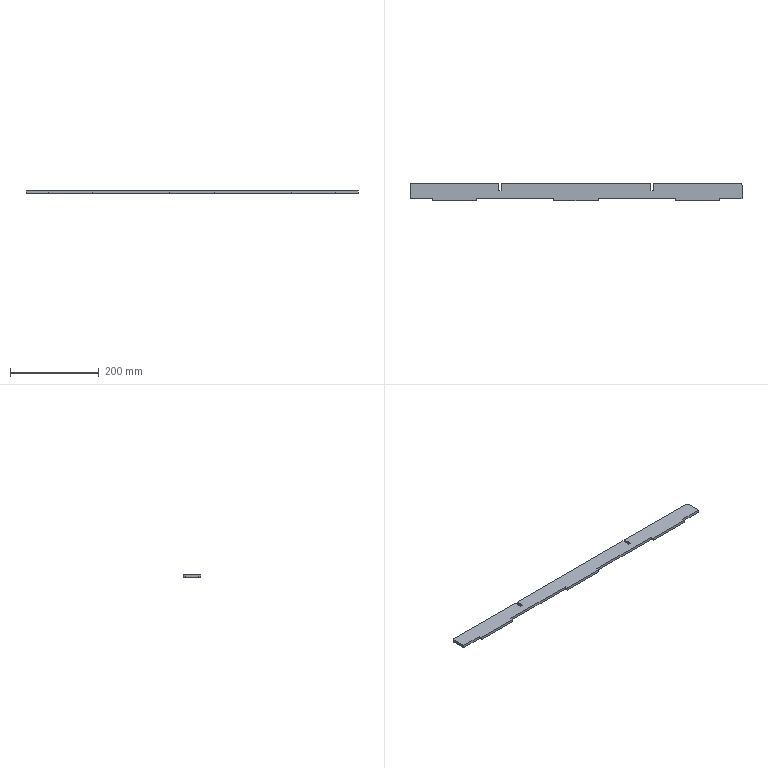Part | SolidWorks | features FlatPattern 1, SMBaseFlange 1, SheetMetal 1 | 1 solid | 28 faces | box 750 x 40.5 x 6 mm | volume 166068 mm3 | plane 26 | cylinder 2 | commonest cylinder face diameters 10 x2
STEP:
#1=CARTESIAN_POINT('',(353.761,-654.3,0.));
#2=VERTEX_POINT('',#1);
#3=CARTESIAN_POINT('',(353.761,-624.3,0.));
#4=VERTEX_POINT('',#3);
#5=CARTESIAN_POINT('',(353.761,-654.3,0.));
#6=DIRECTION('',(0.,1.,0.));
#7=VECTOR('',#6,1000.);
#8=LINE('',#5,#7);
#9=EDGE_CURVE('',#2,#4,#8,.T.);
#10=ORIENTED_EDGE('',*,*,#9,.F.);
#11=CARTESIAN_POINT('',(353.761,-654.3,-6.));
#12=VERTEX_POINT('',#11);
#13=CARTESIAN_POINT('',(353.761,-654.3,-6.));
#14=DIRECTION('',(0.,0.,1.));
#15=VECTOR('',#14,1000.);
#16=LINE('',#13,#15);
#17=EDGE_CURVE('',#12,#2,#16,.T.);
#18=ORIENTED_EDGE('',*,*,#17,.F.);
#19=CARTESIAN_POINT('',(353.761,-624.3,-6.));
#20=VERTEX_POINT('',#19);
#21=CARTESIAN_POINT('',(353.761,-654.3,-6.));
#22=DIRECTION('',(0.,1.,0.));
#23=VECTOR('',#22,1000.);
#24=LINE('',#21,#23);
#25=EDGE_CURVE('',#12,#20,#24,.T.);
#26=ORIENTED_EDGE('',*,*,#25,.T.);
#27=CARTESIAN_POINT('',(353.761,-624.3,-6.));
#28=DIRECTION('',(0.,0.,1.));
#29=VECTOR('',#28,1000.);
#30=LINE('',#27,#29);
#31=EDGE_CURVE('',#20,#4,#30,.T.);
#32=ORIENTED_EDGE('',*,*,#31,.T.);
#33=EDGE_LOOP('',(#10,#18,#26,#32));
#34=FACE_OUTER_BOUND('',#33,.T.);
#35=CARTESIAN_POINT('',(353.761,-654.3,-6.));
#36=DIRECTION('',(1.,0.,0.));
#37=DIRECTION('',(0.,0.,-1.));
#38=AXIS2_PLACEMENT_3D('',#35,#36,#37);
#39=PLANE('',#38);
#40=ADVANCED_FACE('',(#34),#39,.T.);
#41=CARTESIAN_POINT('',(303.761,-654.3,0.));
#42=VERTEX_POINT('',#41);
#43=CARTESIAN_POINT('',(353.761,-654.3,0.));
#44=DIRECTION('',(1.,0.,0.));
#45=VECTOR('',#44,1000.);
#46=LINE('',#43,#45);
#47=EDGE_CURVE('',#42,#2,#46,.T.);
#48=ORIENTED_EDGE('',*,*,#47,.F.);
#49=CARTESIAN_POINT('',(303.761,-654.3,-6.));
#50=VERTEX_POINT('',#49);
#51=CARTESIAN_POINT('',(303.761,-654.3,-6.));
#52=DIRECTION('',(0.,0.,1.));
#53=VECTOR('',#52,1000.);
#54=LINE('',#51,#53);
#55=EDGE_CURVE('',#50,#42,#54,.T.);
#56=ORIENTED_EDGE('',*,*,#55,.F.);
#57=CARTESIAN_POINT('',(353.761,-654.3,-6.));
#58=DIRECTION('',(1.,0.,0.));
#59=VECTOR('',#58,1000.);
#60=LINE('',#57,#59);
#61=EDGE_CURVE('',#50,#12,#60,.T.);
#62=ORIENTED_EDGE('',*,*,#61,.T.);
#63=ORIENTED_EDGE('',*,*,#17,.T.);
#64=EDGE_LOOP('',(#48,#56,#62,#63));
#65=FACE_OUTER_BOUND('',#64,.T.);
#66=CARTESIAN_POINT('',(353.761,-654.3,-6.));
#67=DIRECTION('',(0.,-1.,0.));
#68=DIRECTION('',(0.,0.,-1.));
#69=AXIS2_PLACEMENT_3D('',#66,#67,#68);
#70=PLANE('',#69);
#71=ADVANCED_FACE('',(#65),#70,.T.);
#72=CARTESIAN_POINT('',(303.761,-659.8,0.));
#73=VERTEX_POINT('',#72);
#74=CARTESIAN_POINT('',(303.761,-654.3,0.));
#75=DIRECTION('',(0.,1.,0.));
#76=VECTOR('',#75,1000.);
#77=LINE('',#74,#76);
#78=EDGE_CURVE('',#73,#42,#77,.T.);
#79=ORIENTED_EDGE('',*,*,#78,.F.);
#80=CARTESIAN_POINT('',(303.761,-659.8,-6.));
#81=VERTEX_POINT('',#80);
#82=CARTESIAN_POINT('',(303.761,-659.8,-6.));
#83=DIRECTION('',(0.,0.,1.));
#84=VECTOR('',#83,1000.);
#85=LINE('',#82,#84);
#86=EDGE_CURVE('',#81,#73,#85,.T.);
#87=ORIENTED_EDGE('',*,*,#86,.F.);
#88=CARTESIAN_POINT('',(303.761,-654.3,-6.));
#89=DIRECTION('',(0.,1.,0.));
#90=VECTOR('',#89,1000.);
#91=LINE('',#88,#90);
#92=EDGE_CURVE('',#81,#50,#91,.T.);
#93=ORIENTED_EDGE('',*,*,#92,.T.);
#94=ORIENTED_EDGE('',*,*,#55,.T.);
#95=EDGE_LOOP('',(#79,#87,#93,#94));
#96=FACE_OUTER_BOUND('',#95,.T.);
#97=CARTESIAN_POINT('',(303.761,-654.3,-6.));
#98=DIRECTION('',(1.,0.,0.));
#99=DIRECTION('',(0.,0.,-1.));
#100=AXIS2_PLACEMENT_3D('',#97,#98,#99);
#101=PLANE('',#100);
#102=ADVANCED_FACE('',(#96),#101,.T.);
#103=CARTESIAN_POINT('',(203.761,-659.8,0.));
#104=VERTEX_POINT('',#103);
#105=CARTESIAN_POINT('',(303.761,-659.8,0.));
#106=DIRECTION('',(1.,0.,0.));
#107=VECTOR('',#106,1000.);
#108=LINE('',#105,#107);
#109=EDGE_CURVE('',#104,#73,#108,.T.);
#110=ORIENTED_EDGE('',*,*,#109,.F.);
#111=CARTESIAN_POINT('',(203.761,-659.8,-6.));
#112=VERTEX_POINT('',#111);
#113=CARTESIAN_POINT('',(203.761,-659.8,-6.));
#114=DIRECTION('',(0.,0.,1.));
#115=VECTOR('',#114,1000.);
#116=LINE('',#113,#115);
#117=EDGE_CURVE('',#112,#104,#116,.T.);
#118=ORIENTED_EDGE('',*,*,#117,.F.);
#119=CARTESIAN_POINT('',(303.761,-659.8,-6.));
#120=DIRECTION('',(1.,0.,0.));
#121=VECTOR('',#120,1000.);
#122=LINE('',#119,#121);
#123=EDGE_CURVE('',#112,#81,#122,.T.);
#124=ORIENTED_EDGE('',*,*,#123,.T.);
#125=ORIENTED_EDGE('',*,*,#86,.T.);
#126=EDGE_LOOP('',(#110,#118,#124,#125));
#127=FACE_OUTER_BOUND('',#126,.T.);
#128=CARTESIAN_POINT('',(303.761,-659.8,-6.));
#129=DIRECTION('',(0.,-1.,0.));
#130=DIRECTION('',(1.,0.,0.));
#131=AXIS2_PLACEMENT_3D('',#128,#129,#130);
#132=PLANE('',#131);
#133=ADVANCED_FACE('',(#127),#132,.T.);
#134=CARTESIAN_POINT('',(203.761,-654.3,0.));
#135=VERTEX_POINT('',#134);
#136=CARTESIAN_POINT('',(203.761,-659.8,0.));
#137=DIRECTION('',(0.,-1.,0.));
#138=VECTOR('',#137,1000.);
#139=LINE('',#136,#138);
#140=EDGE_CURVE('',#135,#104,#139,.T.);
#141=ORIENTED_EDGE('',*,*,#140,.F.);
#142=CARTESIAN_POINT('',(203.761,-654.3,-6.));
#143=VERTEX_POINT('',#142);
#144=CARTESIAN_POINT('',(203.761,-654.3,-6.));
#145=DIRECTION('',(0.,0.,1.));
#146=VECTOR('',#145,1000.);
#147=LINE('',#144,#146);
#148=EDGE_CURVE('',#143,#135,#147,.T.);
#149=ORIENTED_EDGE('',*,*,#148,.F.);
#150=CARTESIAN_POINT('',(203.761,-659.8,-6.));
#151=DIRECTION('',(0.,-1.,0.));
#152=VECTOR('',#151,1000.);
#153=LINE('',#150,#152);
#154=EDGE_CURVE('',#143,#112,#153,.T.);
#155=ORIENTED_EDGE('',*,*,#154,.T.);
#156=ORIENTED_EDGE('',*,*,#117,.T.);
#157=EDGE_LOOP('',(#141,#149,#155,#156));
#158=FACE_OUTER_BOUND('',#157,.T.);
#159=CARTESIAN_POINT('',(203.761,-659.8,-6.));
#160=DIRECTION('',(-1.,0.,0.));
#161=DIRECTION('',(0.,0.,1.));
#162=AXIS2_PLACEMENT_3D('',#159,#160,#161);
#163=PLANE('',#162);
#164=ADVANCED_FACE('',(#158),#163,.T.);
#165=CARTESIAN_POINT('',(28.761,-654.3,0.));
#166=VERTEX_POINT('',#165);
#167=CARTESIAN_POINT('',(203.761,-654.3,0.));
#168=DIRECTION('',(1.,0.,0.));
#169=VECTOR('',#168,1000.);
#170=LINE('',#167,#169);
#171=EDGE_CURVE('',#166,#135,#170,.T.);
#172=ORIENTED_EDGE('',*,*,#171,.F.);
#173=CARTESIAN_POINT('',(28.761,-654.3,-6.));
#174=VERTEX_POINT('',#173);
#175=CARTESIAN_POINT('',(28.761,-654.3,-6.));
#176=DIRECTION('',(0.,0.,1.));
#177=VECTOR('',#176,1000.);
#178=LINE('',#175,#177);
#179=EDGE_CURVE('',#174,#166,#178,.T.);
#180=ORIENTED_EDGE('',*,*,#179,.F.);
#181=CARTESIAN_POINT('',(203.761,-654.3,-6.));
#182=DIRECTION('',(1.,0.,0.));
#183=VECTOR('',#182,1000.);
#184=LINE('',#181,#183);
#185=EDGE_CURVE('',#174,#143,#184,.T.);
#186=ORIENTED_EDGE('',*,*,#185,.T.);
#187=ORIENTED_EDGE('',*,*,#148,.T.);
#188=EDGE_LOOP('',(#172,#180,#186,#187));
#189=FACE_OUTER_BOUND('',#188,.T.);
#190=CARTESIAN_POINT('',(203.761,-654.3,-6.));
#191=DIRECTION('',(0.,-1.,0.));
#192=DIRECTION('',(0.,0.,-1.));
#193=AXIS2_PLACEMENT_3D('',#190,#191,#192);
#194=PLANE('',#193);
#195=ADVANCED_FACE('',(#189),#194,.T.);
#196=CARTESIAN_POINT('',(28.761,-659.8,0.));
#197=VERTEX_POINT('',#196);
#198=CARTESIAN_POINT('',(28.761,-654.3,0.));
#199=DIRECTION('',(0.,1.,0.));
#200=VECTOR('',#199,1000.);
#201=LINE('',#198,#200);
#202=EDGE_CURVE('',#197,#166,#201,.T.);
#203=ORIENTED_EDGE('',*,*,#202,.F.);
#204=CARTESIAN_POINT('',(28.761,-659.8,-6.));
#205=VERTEX_POINT('',#204);
#206=CARTESIAN_POINT('',(28.761,-659.8,-6.));
#207=DIRECTION('',(0.,0.,1.));
#208=VECTOR('',#207,1000.);
#209=LINE('',#206,#208);
#210=EDGE_CURVE('',#205,#197,#209,.T.);
#211=ORIENTED_EDGE('',*,*,#210,.F.);
#212=CARTESIAN_POINT('',(28.761,-654.3,-6.));
#213=DIRECTION('',(0.,1.,0.));
#214=VECTOR('',#213,1000.);
#215=LINE('',#212,#214);
#216=EDGE_CURVE('',#205,#174,#215,.T.);
#217=ORIENTED_EDGE('',*,*,#216,.T.);
#218=ORIENTED_EDGE('',*,*,#179,.T.);
#219=EDGE_LOOP('',(#203,#211,#217,#218));
#220=FACE_OUTER_BOUND('',#219,.T.);
#221=CARTESIAN_POINT('',(28.761,-654.3,-6.));
#222=DIRECTION('',(1.,0.,0.));
#223=DIRECTION('',(0.,1.,0.));
#224=AXIS2_PLACEMENT_3D('',#221,#222,#223);
#225=PLANE('',#224);
#226=ADVANCED_FACE('',(#220),#225,.T.);
#227=CARTESIAN_POINT('',(-71.239,-659.8,0.));
#228=VERTEX_POINT('',#227);
#229=CARTESIAN_POINT('',(28.761,-659.8,0.));
#230=DIRECTION('',(1.,0.,0.));
#231=VECTOR('',#230,1000.);
#232=LINE('',#229,#231);
#233=EDGE_CURVE('',#228,#197,#232,.T.);
#234=ORIENTED_EDGE('',*,*,#233,.F.);
#235=CARTESIAN_POINT('',(-71.239,-659.8,-6.));
#236=VERTEX_POINT('',#235);
#237=CARTESIAN_POINT('',(-71.239,-659.8,-6.));
#238=DIRECTION('',(0.,0.,1.));
#239=VECTOR('',#238,1000.);
#240=LINE('',#237,#239);
#241=EDGE_CURVE('',#236,#228,#240,.T.);
#242=ORIENTED_EDGE('',*,*,#241,.F.);
#243=CARTESIAN_POINT('',(28.761,-659.8,-6.));
#244=DIRECTION('',(1.,0.,0.));
#245=VECTOR('',#244,1000.);
#246=LINE('',#243,#245);
#247=EDGE_CURVE('',#236,#205,#246,.T.);
#248=ORIENTED_EDGE('',*,*,#247,.T.);
#249=ORIENTED_EDGE('',*,*,#210,.T.);
#250=EDGE_LOOP('',(#234,#242,#248,#249));
#251=FACE_OUTER_BOUND('',#250,.T.);
#252=CARTESIAN_POINT('',(28.761,-659.8,-6.));
#253=DIRECTION('',(0.,-1.,0.));
#254=DIRECTION('',(0.,0.,-1.));
#255=AXIS2_PLACEMENT_3D('',#252,#253,#254);
#256=PLANE('',#255);
#257=ADVANCED_FACE('',(#251),#256,.T.);
#258=CARTESIAN_POINT('',(-71.239,-654.3,0.));
#259=VERTEX_POINT('',#258);
#260=CARTESIAN_POINT('',(-71.239,-659.8,0.));
#261=DIRECTION('',(0.,-1.,0.));
#262=VECTOR('',#261,1000.);
#263=LINE('',#260,#262);
#264=EDGE_CURVE('',#259,#228,#263,.T.);
#265=ORIENTED_EDGE('',*,*,#264,.F.);
#266=CARTESIAN_POINT('',(-71.239,-654.3,-6.));
#267=VERTEX_POINT('',#266);
#268=CARTESIAN_POINT('',(-71.239,-654.3,-6.));
#269=DIRECTION('',(0.,0.,1.));
#270=VECTOR('',#269,1000.);
#271=LINE('',#268,#270);
#272=EDGE_CURVE('',#267,#259,#271,.T.);
#273=ORIENTED_EDGE('',*,*,#272,.F.);
#274=CARTESIAN_POINT('',(-71.239,-659.8,-6.));
#275=DIRECTION('',(0.,-1.,0.));
#276=VECTOR('',#275,1000.);
#277=LINE('',#274,#276);
#278=EDGE_CURVE('',#267,#236,#277,.T.);
#279=ORIENTED_EDGE('',*,*,#278,.T.);
#280=ORIENTED_EDGE('',*,*,#241,.T.);
#281=EDGE_LOOP('',(#265,#273,#279,#280));
#282=FACE_OUTER_BOUND('',#281,.T.);
#283=CARTESIAN_POINT('',(-71.239,-659.8,-6.));
#284=DIRECTION('',(-1.,0.,0.));
#285=DIRECTION('',(0.,-1.,0.));
#286=AXIS2_PLACEMENT_3D('',#283,#284,#285);
#287=PLANE('',#286);
#288=ADVANCED_FACE('',(#282),#287,.T.);
#289=CARTESIAN_POINT('',(-246.239,-654.3,0.));
#290=VERTEX_POINT('',#289);
#291=CARTESIAN_POINT('',(-71.239,-654.3,0.));
#292=DIRECTION('',(1.,0.,0.));
#293=VECTOR('',#292,1000.);
#294=LINE('',#291,#293);
#295=EDGE_CURVE('',#290,#259,#294,.T.);
#296=ORIENTED_EDGE('',*,*,#295,.F.);
#297=CARTESIAN_POINT('',(-246.239,-654.3,-6.));
#298=VERTEX_POINT('',#297);
#299=CARTESIAN_POINT('',(-246.239,-654.3,-6.));
#300=DIRECTION('',(0.,0.,1.));
#301=VECTOR('',#300,1000.);
#302=LINE('',#299,#301);
#303=EDGE_CURVE('',#298,#290,#302,.T.);
#304=ORIENTED_EDGE('',*,*,#303,.F.);
#305=CARTESIAN_POINT('',(-71.239,-654.3,-6.));
#306=DIRECTION('',(1.,0.,0.));
#307=VECTOR('',#306,1000.);
#308=LINE('',#305,#307);
#309=EDGE_CURVE('',#298,#267,#308,.T.);
#310=ORIENTED_EDGE('',*,*,#309,.T.);
#311=ORIENTED_EDGE('',*,*,#272,.T.);
#312=EDGE_LOOP('',(#296,#304,#310,#311));
#313=FACE_OUTER_BOUND('',#312,.T.);
#314=CARTESIAN_POINT('',(-71.239,-654.3,-6.));
#315=DIRECTION('',(0.,-1.,0.));
#316=DIRECTION('',(1.,0.,0.));
#317=AXIS2_PLACEMENT_3D('',#314,#315,#316);
#318=PLANE('',#317);
#319=ADVANCED_FACE('',(#313),#318,.T.);
#320=CARTESIAN_POINT('',(-246.239,-659.8,0.));
#321=VERTEX_POINT('',#320);
#322=CARTESIAN_POINT('',(-246.239,-659.8,0.));
#323=DIRECTION('',(0.,1.,0.));
#324=VECTOR('',#323,1000.);
#325=LINE('',#322,#324);
#326=EDGE_CURVE('',#321,#290,#325,.T.);
#327=ORIENTED_EDGE('',*,*,#326,.F.);
#328=CARTESIAN_POINT('',(-246.239,-659.8,-6.));
#329=VERTEX_POINT('',#328);
#330=CARTESIAN_POINT('',(-246.239,-659.8,-6.));
#331=DIRECTION('',(0.,0.,1.));
#332=VECTOR('',#331,1000.);
#333=LINE('',#330,#332);
#334=EDGE_CURVE('',#329,#321,#333,.T.);
#335=ORIENTED_EDGE('',*,*,#334,.F.);
#336=CARTESIAN_POINT('',(-246.239,-659.8,-6.));
#337=DIRECTION('',(0.,1.,0.));
#338=VECTOR('',#337,1000.);
#339=LINE('',#336,#338);
#340=EDGE_CURVE('',#329,#298,#339,.T.);
#341=ORIENTED_EDGE('',*,*,#340,.T.);
#342=ORIENTED_EDGE('',*,*,#303,.T.);
#343=EDGE_LOOP('',(#327,#335,#341,#342));
#344=FACE_OUTER_BOUND('',#343,.T.);
#345=CARTESIAN_POINT('',(-246.239,-659.8,-6.));
#346=DIRECTION('',(1.,0.,0.));
#347=DIRECTION('',(0.,0.,-1.));
#348=AXIS2_PLACEMENT_3D('',#345,#346,#347);
#349=PLANE('',#348);
#350=ADVANCED_FACE('',(#344),#349,.T.);
#351=CARTESIAN_POINT('',(-346.239,-659.8,0.));
#352=VERTEX_POINT('',#351);
#353=CARTESIAN_POINT('',(-346.239,-659.8,0.));
#354=DIRECTION('',(1.,0.,0.));
#355=VECTOR('',#354,1000.);
#356=LINE('',#353,#355);
#357=EDGE_CURVE('',#352,#321,#356,.T.);
#358=ORIENTED_EDGE('',*,*,#357,.F.);
#359=CARTESIAN_POINT('',(-346.239,-659.8,-6.));
#360=VERTEX_POINT('',#359);
#361=CARTESIAN_POINT('',(-346.239,-659.8,-6.));
#362=DIRECTION('',(0.,0.,1.));
#363=VECTOR('',#362,1000.);
#364=LINE('',#361,#363);
#365=EDGE_CURVE('',#360,#352,#364,.T.);
#366=ORIENTED_EDGE('',*,*,#365,.F.);
#367=CARTESIAN_POINT('',(-346.239,-659.8,-6.));
#368=DIRECTION('',(1.,0.,0.));
#369=VECTOR('',#368,1000.);
#370=LINE('',#367,#369);
#371=EDGE_CURVE('',#360,#329,#370,.T.);
#372=ORIENTED_EDGE('',*,*,#371,.T.);
#373=ORIENTED_EDGE('',*,*,#334,.T.);
#374=EDGE_LOOP('',(#358,#366,#372,#373));
#375=FACE_OUTER_BOUND('',#374,.T.);
#376=CARTESIAN_POINT('',(-346.239,-659.8,-6.));
#377=DIRECTION('',(0.,-1.,0.));
#378=DIRECTION('',(0.,0.,-1.));
#379=AXIS2_PLACEMENT_3D('',#376,#377,#378);
#380=PLANE('',#379);
#381=ADVANCED_FACE('',(#375),#380,.T.);
#382=CARTESIAN_POINT('',(-346.239,-654.3,0.));
#383=VERTEX_POINT('',#382);
#384=CARTESIAN_POINT('',(-346.239,-654.3,0.));
#385=DIRECTION('',(0.,-1.,0.));
#386=VECTOR('',#385,1000.);
#387=LINE('',#384,#386);
#388=EDGE_CURVE('',#383,#352,#387,.T.);
#389=ORIENTED_EDGE('',*,*,#388,.F.);
#390=CARTESIAN_POINT('',(-346.239,-654.3,-6.));
#391=VERTEX_POINT('',#390);
#392=CARTESIAN_POINT('',(-346.239,-654.3,-6.));
#393=DIRECTION('',(0.,0.,1.));
#394=VECTOR('',#393,1000.);
#395=LINE('',#392,#394);
#396=EDGE_CURVE('',#391,#383,#395,.T.);
#397=ORIENTED_EDGE('',*,*,#396,.F.);
#398=CARTESIAN_POINT('',(-346.239,-654.3,-6.));
#399=DIRECTION('',(0.,-1.,0.));
#400=VECTOR('',#399,1000.);
#401=LINE('',#398,#400);
#402=EDGE_CURVE('',#391,#360,#401,.T.);
#403=ORIENTED_EDGE('',*,*,#402,.T.);
#404=ORIENTED_EDGE('',*,*,#365,.T.);
#405=EDGE_LOOP('',(#389,#397,#403,#404));
#406=FACE_OUTER_BOUND('',#405,.T.);
#407=CARTESIAN_POINT('',(-346.239,-654.3,-6.));
#408=DIRECTION('',(-1.,0.,0.));
#409=DIRECTION('',(0.,0.,1.));
#410=AXIS2_PLACEMENT_3D('',#407,#408,#409);
#411=PLANE('',#410);
#412=ADVANCED_FACE('',(#406),#411,.T.);
#413=CARTESIAN_POINT('',(-396.239,-654.3,0.));
#414=VERTEX_POINT('',#413);
#415=CARTESIAN_POINT('',(-346.239,-654.3,0.));
#416=DIRECTION('',(1.,0.,0.));
#417=VECTOR('',#416,1000.);
#418=LINE('',#415,#417);
#419=EDGE_CURVE('',#414,#383,#418,.T.);
#420=ORIENTED_EDGE('',*,*,#419,.F.);
#421=CARTESIAN_POINT('',(-396.239,-654.3,-6.));
#422=VERTEX_POINT('',#421);
#423=CARTESIAN_POINT('',(-396.239,-654.3,-6.));
#424=DIRECTION('',(0.,0.,1.));
#425=VECTOR('',#424,1000.);
#426=LINE('',#423,#425);
#427=EDGE_CURVE('',#422,#414,#426,.T.);
#428=ORIENTED_EDGE('',*,*,#427,.F.);
#429=CARTESIAN_POINT('',(-346.239,-654.3,-6.));
#430=DIRECTION('',(1.,0.,0.));
#431=VECTOR('',#430,1000.);
#432=LINE('',#429,#431);
#433=EDGE_CURVE('',#422,#391,#432,.T.);
#434=ORIENTED_EDGE('',*,*,#433,.T.);
#435=ORIENTED_EDGE('',*,*,#396,.T.);
#436=EDGE_LOOP('',(#420,#428,#434,#435));
#437=FACE_OUTER_BOUND('',#436,.T.);
#438=CARTESIAN_POINT('',(-346.239,-654.3,-6.));
#439=DIRECTION('',(0.,-1.,0.));
#440=DIRECTION('',(1.,0.,0.));
#441=AXIS2_PLACEMENT_3D('',#438,#439,#440);
#442=PLANE('',#441);
#443=ADVANCED_FACE('',(#437),#442,.T.);
#444=CARTESIAN_POINT('',(-396.239,-624.3,0.));
#445=VERTEX_POINT('',#444);
#446=CARTESIAN_POINT('',(-396.239,-654.3,0.));
#447=DIRECTION('',(0.,-1.,0.));
#448=VECTOR('',#447,1000.);
#449=LINE('',#446,#448);
#450=EDGE_CURVE('',#445,#414,#449,.T.);
#451=ORIENTED_EDGE('',*,*,#450,.F.);
#452=CARTESIAN_POINT('',(-396.239,-624.3,-6.));
#453=VERTEX_POINT('',#452);
#454=CARTESIAN_POINT('',(-396.239,-624.3,-6.));
#455=DIRECTION('',(0.,0.,1.));
#456=VECTOR('',#455,1000.);
#457=LINE('',#454,#456);
#458=EDGE_CURVE('',#453,#445,#457,.T.);
#459=ORIENTED_EDGE('',*,*,#458,.F.);
#460=CARTESIAN_POINT('',(-396.239,-654.3,-6.));
#461=DIRECTION('',(0.,-1.,0.));
#462=VECTOR('',#461,1000.);
#463=LINE('',#460,#462);
#464=EDGE_CURVE('',#453,#422,#463,.T.);
#465=ORIENTED_EDGE('',*,*,#464,.T.);
#466=ORIENTED_EDGE('',*,*,#427,.T.);
#467=EDGE_LOOP('',(#451,#459,#465,#466));
#468=FACE_OUTER_BOUND('',#467,.T.);
#469=CARTESIAN_POINT('',(-396.239,-654.3,-6.));
#470=DIRECTION('',(-1.,0.,0.));
#471=DIRECTION('',(0.,0.,1.));
#472=AXIS2_PLACEMENT_3D('',#469,#470,#471);
#473=PLANE('',#472);
#474=ADVANCED_FACE('',(#468),#473,.T.);
#475=CARTESIAN_POINT('',(-391.239,-619.3,0.));
#476=VERTEX_POINT('',#475);
#477=CARTESIAN_POINT('',(-391.239,-624.3,0.));
#478=DIRECTION('',(0.,0.,1.));
#479=DIRECTION('',(1.,0.,0.));
#480=AXIS2_PLACEMENT_3D('',#477,#478,#479);
#481=CIRCLE('',#480,5.);
#482=EDGE_CURVE('',#476,#445,#481,.T.);
#483=ORIENTED_EDGE('',*,*,#482,.F.);
#484=CARTESIAN_POINT('',(-391.239,-619.3,-6.));
#485=VERTEX_POINT('',#484);
#486=CARTESIAN_POINT('',(-391.239,-619.3,-6.));
#487=DIRECTION('',(0.,0.,1.));
#488=VECTOR('',#487,1000.);
#489=LINE('',#486,#488);
#490=EDGE_CURVE('',#485,#476,#489,.T.);
#491=ORIENTED_EDGE('',*,*,#490,.F.);
#492=CARTESIAN_POINT('',(-391.239,-624.3,-6.));
#493=DIRECTION('',(0.,0.,1.));
#494=DIRECTION('',(1.,0.,0.));
#495=AXIS2_PLACEMENT_3D('',#492,#493,#494);
#496=CIRCLE('',#495,5.);
#497=EDGE_CURVE('',#485,#453,#496,.T.);
#498=ORIENTED_EDGE('',*,*,#497,.T.);
#499=ORIENTED_EDGE('',*,*,#458,.T.);
#500=EDGE_LOOP('',(#483,#491,#498,#499));
#501=FACE_OUTER_BOUND('',#500,.T.);
#502=CARTESIAN_POINT('',(-391.239,-624.3,-6.));
#503=DIRECTION('',(0.,0.,1.));
#504=DIRECTION('',(1.,0.,0.));
#505=AXIS2_PLACEMENT_3D('',#502,#503,#504);
#506=CYLINDRICAL_SURFACE('',#505,5.);
#507=ADVANCED_FACE('',(#501),#506,.T.);
#508=CARTESIAN_POINT('',(-196.239,-619.3,0.));
#509=VERTEX_POINT('',#508);
#510=CARTESIAN_POINT('',(-196.239,-619.3,0.));
#511=DIRECTION('',(-1.,0.,0.));
#512=VECTOR('',#511,1000.);
#513=LINE('',#510,#512);
#514=EDGE_CURVE('',#509,#476,#513,.T.);
#515=ORIENTED_EDGE('',*,*,#514,.F.);
#516=CARTESIAN_POINT('',(-196.239,-619.3,-6.));
#517=VERTEX_POINT('',#516);
#518=CARTESIAN_POINT('',(-196.239,-619.3,-6.));
#519=DIRECTION('',(0.,0.,1.));
#520=VECTOR('',#519,1000.);
#521=LINE('',#518,#520);
#522=EDGE_CURVE('',#517,#509,#521,.T.);
#523=ORIENTED_EDGE('',*,*,#522,.F.);
#524=CARTESIAN_POINT('',(-196.239,-619.3,-6.));
#525=DIRECTION('',(-1.,0.,0.));
#526=VECTOR('',#525,1000.);
#527=LINE('',#524,#526);
#528=EDGE_CURVE('',#517,#485,#527,.T.);
#529=ORIENTED_EDGE('',*,*,#528,.T.);
#530=ORIENTED_EDGE('',*,*,#490,.T.);
#531=EDGE_LOOP('',(#515,#523,#529,#530));
#532=FACE_OUTER_BOUND('',#531,.T.);
#533=CARTESIAN_POINT('',(-196.239,-619.3,-6.));
#534=DIRECTION('',(0.,1.,0.));
#535=DIRECTION('',(0.,0.,1.));
#536=AXIS2_PLACEMENT_3D('',#533,#534,#535);
#537=PLANE('',#536);
#538=ADVANCED_FACE('',(#532),#537,.T.);
#539=CARTESIAN_POINT('',(-196.239,-636.9,0.));
#540=VERTEX_POINT('',#539);
#541=CARTESIAN_POINT('',(-196.239,-636.9,0.));
#542=DIRECTION('',(0.,1.,0.));
#543=VECTOR('',#542,1000.);
#544=LINE('',#541,#543);
#545=EDGE_CURVE('',#540,#509,#544,.T.);
#546=ORIENTED_EDGE('',*,*,#545,.F.);
#547=CARTESIAN_POINT('',(-196.239,-636.9,-6.));
#548=VERTEX_POINT('',#547);
#549=CARTESIAN_POINT('',(-196.239,-636.9,-6.));
#550=DIRECTION('',(0.,0.,1.));
#551=VECTOR('',#550,1000.);
#552=LINE('',#549,#551);
#553=EDGE_CURVE('',#548,#540,#552,.T.);
#554=ORIENTED_EDGE('',*,*,#553,.F.);
#555=CARTESIAN_POINT('',(-196.239,-636.9,-6.));
#556=DIRECTION('',(0.,1.,0.));
#557=VECTOR('',#556,1000.);
#558=LINE('',#555,#557);
#559=EDGE_CURVE('',#548,#517,#558,.T.);
#560=ORIENTED_EDGE('',*,*,#559,.T.);
#561=ORIENTED_EDGE('',*,*,#522,.T.);
#562=EDGE_LOOP('',(#546,#554,#560,#561));
#563=FACE_OUTER_BOUND('',#562,.T.);
#564=CARTESIAN_POINT('',(-196.239,-636.9,-6.));
#565=DIRECTION('',(1.,0.,0.));
#566=DIRECTION('',(0.,1.,0.));
#567=AXIS2_PLACEMENT_3D('',#564,#565,#566);
#568=PLANE('',#567);
#569=ADVANCED_FACE('',(#563),#568,.T.);
#570=CARTESIAN_POINT('',(-190.239,-636.9,0.));
#571=VERTEX_POINT('',#570);
#572=CARTESIAN_POINT('',(-190.239,-636.9,0.));
#573=DIRECTION('',(-1.,0.,0.));
#574=VECTOR('',#573,1000.);
#575=LINE('',#572,#574);
#576=EDGE_CURVE('',#571,#540,#575,.T.);
#577=ORIENTED_EDGE('',*,*,#576,.F.);
#578=CARTESIAN_POINT('',(-190.239,-636.9,-6.));
#579=VERTEX_POINT('',#578);
#580=CARTESIAN_POINT('',(-190.239,-636.9,-6.));
#581=DIRECTION('',(0.,0.,1.));
#582=VECTOR('',#581,1000.);
#583=LINE('',#580,#582);
#584=EDGE_CURVE('',#579,#571,#583,.T.);
#585=ORIENTED_EDGE('',*,*,#584,.F.);
#586=CARTESIAN_POINT('',(-190.239,-636.9,-6.));
#587=DIRECTION('',(-1.,0.,0.));
#588=VECTOR('',#587,1000.);
#589=LINE('',#586,#588);
#590=EDGE_CURVE('',#579,#548,#589,.T.);
#591=ORIENTED_EDGE('',*,*,#590,.T.);
#592=ORIENTED_EDGE('',*,*,#553,.T.);
#593=EDGE_LOOP('',(#577,#585,#591,#592));
#594=FACE_OUTER_BOUND('',#593,.T.);
#595=CARTESIAN_POINT('',(-190.239,-636.9,-6.));
#596=DIRECTION('',(0.,1.,0.));
#597=DIRECTION('',(0.,0.,1.));
#598=AXIS2_PLACEMENT_3D('',#595,#596,#597);
#599=PLANE('',#598);
#600=ADVANCED_FACE('',(#594),#599,.T.);
#601=CARTESIAN_POINT('',(-190.239,-619.3,0.));
#602=VERTEX_POINT('',#601);
#603=CARTESIAN_POINT('',(-190.239,-619.3,0.));
#604=DIRECTION('',(0.,-1.,0.));
#605=VECTOR('',#604,1000.);
#606=LINE('',#603,#605);
#607=EDGE_CURVE('',#602,#571,#606,.T.);
#608=ORIENTED_EDGE('',*,*,#607,.F.);
#609=CARTESIAN_POINT('',(-190.239,-619.3,-6.));
#610=VERTEX_POINT('',#609);
#611=CARTESIAN_POINT('',(-190.239,-619.3,-6.));
#612=DIRECTION('',(0.,0.,1.));
#613=VECTOR('',#612,1000.);
#614=LINE('',#611,#613);
#615=EDGE_CURVE('',#610,#602,#614,.T.);
#616=ORIENTED_EDGE('',*,*,#615,.F.);
#617=CARTESIAN_POINT('',(-190.239,-619.3,-6.));
#618=DIRECTION('',(0.,-1.,0.));
#619=VECTOR('',#618,1000.);
#620=LINE('',#617,#619);
#621=EDGE_CURVE('',#610,#579,#620,.T.);
#622=ORIENTED_EDGE('',*,*,#621,.T.);
#623=ORIENTED_EDGE('',*,*,#584,.T.);
#624=EDGE_LOOP('',(#608,#616,#622,#623));
#625=FACE_OUTER_BOUND('',#624,.T.);
#626=CARTESIAN_POINT('',(-190.239,-619.3,-6.));
#627=DIRECTION('',(-1.,0.,0.));
#628=DIRECTION('',(0.,0.,1.));
#629=AXIS2_PLACEMENT_3D('',#626,#627,#628);
#630=PLANE('',#629);
#631=ADVANCED_FACE('',(#625),#630,.T.);
#632=CARTESIAN_POINT('',(147.761,-619.3,0.));
#633=VERTEX_POINT('',#632);
#634=CARTESIAN_POINT('',(147.761,-619.3,0.));
#635=DIRECTION('',(-1.,0.,0.));
#636=VECTOR('',#635,1000.);
#637=LINE('',#634,#636);
#638=EDGE_CURVE('',#633,#602,#637,.T.);
#639=ORIENTED_EDGE('',*,*,#638,.F.);
#640=CARTESIAN_POINT('',(147.761,-619.3,-6.));
#641=VERTEX_POINT('',#640);
#642=CARTESIAN_POINT('',(147.761,-619.3,-6.));
#643=DIRECTION('',(0.,0.,1.));
#644=VECTOR('',#643,1000.);
#645=LINE('',#642,#644);
#646=EDGE_CURVE('',#641,#633,#645,.T.);
#647=ORIENTED_EDGE('',*,*,#646,.F.);
#648=CARTESIAN_POINT('',(147.761,-619.3,-6.));
#649=DIRECTION('',(-1.,0.,0.));
#650=VECTOR('',#649,1000.);
#651=LINE('',#648,#650);
#652=EDGE_CURVE('',#641,#610,#651,.T.);
#653=ORIENTED_EDGE('',*,*,#652,.T.);
#654=ORIENTED_EDGE('',*,*,#615,.T.);
#655=EDGE_LOOP('',(#639,#647,#653,#654));
#656=FACE_OUTER_BOUND('',#655,.T.);
#657=CARTESIAN_POINT('',(147.761,-619.3,-6.));
#658=DIRECTION('',(0.,1.,0.));
#659=DIRECTION('',(0.,0.,1.));
#660=AXIS2_PLACEMENT_3D('',#657,#658,#659);
#661=PLANE('',#660);
#662=ADVANCED_FACE('',(#656),#661,.T.);
#663=CARTESIAN_POINT('',(147.761,-636.9,0.));
#664=VERTEX_POINT('',#663);
#665=CARTESIAN_POINT('',(147.761,-636.9,0.));
#666=DIRECTION('',(0.,1.,0.));
#667=VECTOR('',#666,1000.);
#668=LINE('',#665,#667);
#669=EDGE_CURVE('',#664,#633,#668,.T.);
#670=ORIENTED_EDGE('',*,*,#669,.F.);
#671=CARTESIAN_POINT('',(147.761,-636.9,-6.));
#672=VERTEX_POINT('',#671);
#673=CARTESIAN_POINT('',(147.761,-636.9,-6.));
#674=DIRECTION('',(0.,0.,1.));
#675=VECTOR('',#674,1000.);
#676=LINE('',#673,#675);
#677=EDGE_CURVE('',#672,#664,#676,.T.);
#678=ORIENTED_EDGE('',*,*,#677,.F.);
#679=CARTESIAN_POINT('',(147.761,-636.9,-6.));
#680=DIRECTION('',(0.,1.,0.));
#681=VECTOR('',#680,1000.);
#682=LINE('',#679,#681);
#683=EDGE_CURVE('',#672,#641,#682,.T.);
#684=ORIENTED_EDGE('',*,*,#683,.T.);
#685=ORIENTED_EDGE('',*,*,#646,.T.);
#686=EDGE_LOOP('',(#670,#678,#684,#685));
#687=FACE_OUTER_BOUND('',#686,.T.);
#688=CARTESIAN_POINT('',(147.761,-636.9,-6.));
#689=DIRECTION('',(1.,0.,0.));
#690=DIRECTION('',(0.,0.,-1.));
#691=AXIS2_PLACEMENT_3D('',#688,#689,#690);
#692=PLANE('',#691);
#693=ADVANCED_FACE('',(#687),#692,.T.);
#694=CARTESIAN_POINT('',(153.761,-636.9,0.));
#695=VERTEX_POINT('',#694);
#696=CARTESIAN_POINT('',(153.761,-636.9,0.));
#697=DIRECTION('',(-1.,0.,0.));
#698=VECTOR('',#697,1000.);
#699=LINE('',#696,#698);
#700=EDGE_CURVE('',#695,#664,#699,.T.);
#701=ORIENTED_EDGE('',*,*,#700,.F.);
#702=CARTESIAN_POINT('',(153.761,-636.9,-6.));
#703=VERTEX_POINT('',#702);
#704=CARTESIAN_POINT('',(153.761,-636.9,-6.));
#705=DIRECTION('',(0.,0.,1.));
#706=VECTOR('',#705,1000.);
#707=LINE('',#704,#706);
#708=EDGE_CURVE('',#703,#695,#707,.T.);
#709=ORIENTED_EDGE('',*,*,#708,.F.);
#710=CARTESIAN_POINT('',(153.761,-636.9,-6.));
#711=DIRECTION('',(-1.,0.,0.));
#712=VECTOR('',#711,1000.);
#713=LINE('',#710,#712);
#714=EDGE_CURVE('',#703,#672,#713,.T.);
#715=ORIENTED_EDGE('',*,*,#714,.T.);
#716=ORIENTED_EDGE('',*,*,#677,.T.);
#717=EDGE_LOOP('',(#701,#709,#715,#716));
#718=FACE_OUTER_BOUND('',#717,.T.);
#719=CARTESIAN_POINT('',(153.761,-636.9,-6.));
#720=DIRECTION('',(0.,1.,0.));
#721=DIRECTION('',(0.,0.,1.));
#722=AXIS2_PLACEMENT_3D('',#719,#720,#721);
#723=PLANE('',#722);
#724=ADVANCED_FACE('',(#718),#723,.T.);
#725=CARTESIAN_POINT('',(153.761,-619.3,0.));
#726=VERTEX_POINT('',#725);
#727=CARTESIAN_POINT('',(153.761,-619.3,0.));
#728=DIRECTION('',(0.,-1.,0.));
#729=VECTOR('',#728,1000.);
#730=LINE('',#727,#729);
#731=EDGE_CURVE('',#726,#695,#730,.T.);
#732=ORIENTED_EDGE('',*,*,#731,.F.);
#733=CARTESIAN_POINT('',(153.761,-619.3,-6.));
#734=VERTEX_POINT('',#733);
#735=CARTESIAN_POINT('',(153.761,-619.3,-6.));
#736=DIRECTION('',(0.,0.,1.));
#737=VECTOR('',#736,1000.);
#738=LINE('',#735,#737);
#739=EDGE_CURVE('',#734,#726,#738,.T.);
#740=ORIENTED_EDGE('',*,*,#739,.F.);
#741=CARTESIAN_POINT('',(153.761,-619.3,-6.));
#742=DIRECTION('',(0.,-1.,0.));
#743=VECTOR('',#742,1000.);
#744=LINE('',#741,#743);
#745=EDGE_CURVE('',#734,#703,#744,.T.);
#746=ORIENTED_EDGE('',*,*,#745,.T.);
#747=ORIENTED_EDGE('',*,*,#708,.T.);
#748=EDGE_LOOP('',(#732,#740,#746,#747));
#749=FACE_OUTER_BOUND('',#748,.T.);
#750=CARTESIAN_POINT('',(153.761,-619.3,-6.));
#751=DIRECTION('',(-1.,0.,0.));
#752=DIRECTION('',(0.,0.,1.));
#753=AXIS2_PLACEMENT_3D('',#750,#751,#752);
#754=PLANE('',#753);
#755=ADVANCED_FACE('',(#749),#754,.T.);
#756=CARTESIAN_POINT('',(348.761,-619.3,0.));
#757=VERTEX_POINT('',#756);
#758=CARTESIAN_POINT('',(348.761,-619.3,0.));
#759=DIRECTION('',(-1.,0.,0.));
#760=VECTOR('',#759,1000.);
#761=LINE('',#758,#760);
#762=EDGE_CURVE('',#757,#726,#761,.T.);
#763=ORIENTED_EDGE('',*,*,#762,.F.);
#764=CARTESIAN_POINT('',(348.761,-619.3,-6.));
#765=VERTEX_POINT('',#764);
#766=CARTESIAN_POINT('',(348.761,-619.3,-6.));
#767=DIRECTION('',(0.,0.,1.));
#768=VECTOR('',#767,1000.);
#769=LINE('',#766,#768);
#770=EDGE_CURVE('',#765,#757,#769,.T.);
#771=ORIENTED_EDGE('',*,*,#770,.F.);
#772=CARTESIAN_POINT('',(348.761,-619.3,-6.));
#773=DIRECTION('',(-1.,0.,0.));
#774=VECTOR('',#773,1000.);
#775=LINE('',#772,#774);
#776=EDGE_CURVE('',#765,#734,#775,.T.);
#777=ORIENTED_EDGE('',*,*,#776,.T.);
#778=ORIENTED_EDGE('',*,*,#739,.T.);
#779=EDGE_LOOP('',(#763,#771,#777,#778));
#780=FACE_OUTER_BOUND('',#779,.T.);
#781=CARTESIAN_POINT('',(348.761,-619.3,-6.));
#782=DIRECTION('',(0.,1.,0.));
#783=DIRECTION('',(-1.,0.,0.));
#784=AXIS2_PLACEMENT_3D('',#781,#782,#783);
#785=PLANE('',#784);
#786=ADVANCED_FACE('',(#780),#785,.T.);
#787=CARTESIAN_POINT('',(348.761,-624.3,0.));
#788=DIRECTION('',(0.,0.,1.));
#789=DIRECTION('',(1.,0.,0.));
#790=AXIS2_PLACEMENT_3D('',#787,#788,#789);
#791=CIRCLE('',#790,5.);
#792=EDGE_CURVE('',#4,#757,#791,.T.);
#793=ORIENTED_EDGE('',*,*,#792,.F.);
#794=ORIENTED_EDGE('',*,*,#31,.F.);
#795=CARTESIAN_POINT('',(348.761,-624.3,-6.));
#796=DIRECTION('',(0.,0.,1.));
#797=DIRECTION('',(1.,0.,0.));
#798=AXIS2_PLACEMENT_3D('',#795,#796,#797);
#799=CIRCLE('',#798,5.);
#800=EDGE_CURVE('',#20,#765,#799,.T.);
#801=ORIENTED_EDGE('',*,*,#800,.T.);
#802=ORIENTED_EDGE('',*,*,#770,.T.);
#803=EDGE_LOOP('',(#793,#794,#801,#802));
#804=FACE_OUTER_BOUND('',#803,.T.);
#805=CARTESIAN_POINT('',(348.761,-624.3,-6.));
#806=DIRECTION('',(0.,0.,1.));
#807=DIRECTION('',(1.,0.,0.));
#808=AXIS2_PLACEMENT_3D('',#805,#806,#807);
#809=CYLINDRICAL_SURFACE('',#808,5.);
#810=ADVANCED_FACE('',(#804),#809,.T.);
#811=ORIENTED_EDGE('',*,*,#25,.F.);
#812=ORIENTED_EDGE('',*,*,#61,.F.);
#813=ORIENTED_EDGE('',*,*,#92,.F.);
#814=ORIENTED_EDGE('',*,*,#123,.F.);
#815=ORIENTED_EDGE('',*,*,#154,.F.);
#816=ORIENTED_EDGE('',*,*,#185,.F.);
#817=ORIENTED_EDGE('',*,*,#216,.F.);
#818=ORIENTED_EDGE('',*,*,#247,.F.);
#819=ORIENTED_EDGE('',*,*,#278,.F.);
#820=ORIENTED_EDGE('',*,*,#309,.F.);
#821=ORIENTED_EDGE('',*,*,#340,.F.);
#822=ORIENTED_EDGE('',*,*,#371,.F.);
#823=ORIENTED_EDGE('',*,*,#402,.F.);
#824=ORIENTED_EDGE('',*,*,#433,.F.);
#825=ORIENTED_EDGE('',*,*,#464,.F.);
#826=ORIENTED_EDGE('',*,*,#497,.F.);
#827=ORIENTED_EDGE('',*,*,#528,.F.);
#828=ORIENTED_EDGE('',*,*,#559,.F.);
#829=ORIENTED_EDGE('',*,*,#590,.F.);
#830=ORIENTED_EDGE('',*,*,#621,.F.);
#831=ORIENTED_EDGE('',*,*,#652,.F.);
#832=ORIENTED_EDGE('',*,*,#683,.F.);
#833=ORIENTED_EDGE('',*,*,#714,.F.);
#834=ORIENTED_EDGE('',*,*,#745,.F.);
#835=ORIENTED_EDGE('',*,*,#776,.F.);
#836=ORIENTED_EDGE('',*,*,#800,.F.);
#837=EDGE_LOOP('',(#811,#812,#813,#814,#815,#816,#817,#818,#819,#820,#821,#822,#823,#824,#825,#826,#827,#828,#829,#830,#831,#832,#833,#834,#835,#836));
#838=FACE_OUTER_BOUND('',#837,.T.);
#839=CARTESIAN_POINT('',(348.761,-624.3,-6.));
#840=DIRECTION('',(0.,0.,1.));
#841=DIRECTION('',(1.,0.,0.));
#842=AXIS2_PLACEMENT_3D('',#839,#840,#841);
#843=PLANE('',#842);
#844=ADVANCED_FACE('',(#838),#843,.F.);
#845=ORIENTED_EDGE('',*,*,#9,.T.);
#846=ORIENTED_EDGE('',*,*,#792,.T.);
#847=ORIENTED_EDGE('',*,*,#762,.T.);
#848=ORIENTED_EDGE('',*,*,#731,.T.);
#849=ORIENTED_EDGE('',*,*,#700,.T.);
#850=ORIENTED_EDGE('',*,*,#669,.T.);
#851=ORIENTED_EDGE('',*,*,#638,.T.);
#852=ORIENTED_EDGE('',*,*,#607,.T.);
#853=ORIENTED_EDGE('',*,*,#576,.T.);
#854=ORIENTED_EDGE('',*,*,#545,.T.);
#855=ORIENTED_EDGE('',*,*,#514,.T.);
#856=ORIENTED_EDGE('',*,*,#482,.T.);
#857=ORIENTED_EDGE('',*,*,#450,.T.);
#858=ORIENTED_EDGE('',*,*,#419,.T.);
#859=ORIENTED_EDGE('',*,*,#388,.T.);
#860=ORIENTED_EDGE('',*,*,#357,.T.);
#861=ORIENTED_EDGE('',*,*,#326,.T.);
#862=ORIENTED_EDGE('',*,*,#295,.T.);
#863=ORIENTED_EDGE('',*,*,#264,.T.);
#864=ORIENTED_EDGE('',*,*,#233,.T.);
#865=ORIENTED_EDGE('',*,*,#202,.T.);
#866=ORIENTED_EDGE('',*,*,#171,.T.);
#867=ORIENTED_EDGE('',*,*,#140,.T.);
#868=ORIENTED_EDGE('',*,*,#109,.T.);
#869=ORIENTED_EDGE('',*,*,#78,.T.);
#870=ORIENTED_EDGE('',*,*,#47,.T.);
#871=EDGE_LOOP('',(#845,#846,#847,#848,#849,#850,#851,#852,#853,#854,#855,#856,#857,#858,#859,#860,#861,#862,#863,#864,#865,#866,#867,#868,#869,#870));
#872=FACE_OUTER_BOUND('',#871,.T.);
#873=CARTESIAN_POINT('',(348.761,-624.3,0.));
#874=DIRECTION('',(0.,0.,1.));
#875=DIRECTION('',(1.,0.,0.));
#876=AXIS2_PLACEMENT_3D('',#873,#874,#875);
#877=PLANE('',#876);
#878=ADVANCED_FACE('',(#872),#877,.T.);
#879=CLOSED_SHELL('',(#40,#71,#102,#133,#164,#195,#226,#257,#288,#319,#350,#381,#412,#443,#474,#507,#538,#569,#600,#631,#662,#693,#724,#755,#786,#810,#844,#878));
#880=MANIFOLD_SOLID_BREP('',#879);
#881=CARTESIAN_POINT('',(0.,0.,0.));
#882=DIRECTION('',(0.,0.,1.));
#883=DIRECTION('',(1.,0.,0.));
#884=AXIS2_PLACEMENT_3D('',#881,#882,#883);
#885=(LENGTH_UNIT()NAMED_UNIT(*)SI_UNIT(.MILLI.,.METRE.));
#886=UNCERTAINTY_MEASURE_WITH_UNIT(LENGTH_MEASURE(0.00001),#885,'','');
#887=(NAMED_UNIT(*)PLANE_ANGLE_UNIT()SI_UNIT($,.RADIAN.));
#888=(NAMED_UNIT(*)SI_UNIT($,.STERADIAN.)SOLID_ANGLE_UNIT());
#889=(GEOMETRIC_REPRESENTATION_CONTEXT(3)GLOBAL_UNCERTAINTY_ASSIGNED_CONTEXT((#886))GLOBAL_UNIT_ASSIGNED_CONTEXT((#885,#887,#888))REPRESENTATION_CONTEXT('',''));
#890=ADVANCED_BREP_SHAPE_REPRESENTATION('',(#880,#884),#889);